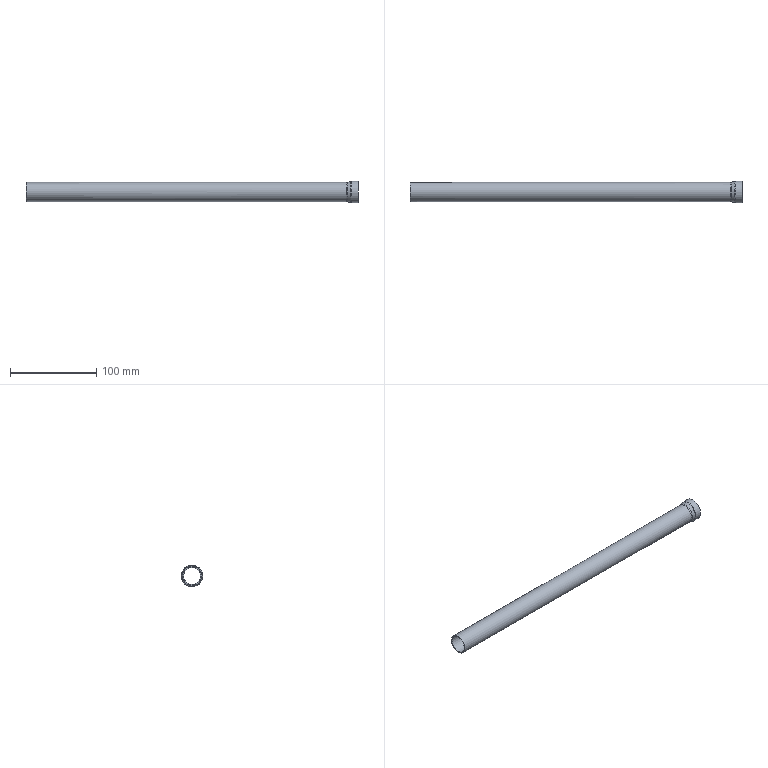Part | NX | features pipe setelah expand 2 | 1 solid | 17 faces | box 385 x 24.9 x 24.9 mm | volume 30600 mm3 | spline 6 | cylinder 4 | torus 3 | plane 2 | cone 2 | commonest cylinder face diameters 19.8 x1 22.2 x1 22.5 x1 24.9 x1
STEP:
#1=CARTESIAN_POINT('',(244.148,128.606,-196.573));
#2=VERTEX_POINT('',#1);
#3=CARTESIAN_POINT('',(244.148,139.394,-176.827));
#4=VERTEX_POINT('',#3);
#5=CARTESIAN_POINT('',(244.148,134.,-186.7));
#6=DIRECTION('',(1.,0.,0.));
#7=DIRECTION('',(0.,1.,0.));
#8=AXIS2_PLACEMENT_3D('',#5,#6,#7);
#9=CIRCLE('',#8,11.25);
#10=EDGE_CURVE('',#2,#4,#9,.T.);
#11=ORIENTED_EDGE('',*,*,#10,.F.);
#12=CARTESIAN_POINT('',(244.148,134.,-186.7));
#13=DIRECTION('',(1.,0.,0.));
#14=DIRECTION('',(0.,1.,0.));
#15=AXIS2_PLACEMENT_3D('',#12,#13,#14);
#16=CIRCLE('',#15,11.25);
#17=EDGE_CURVE('',#4,#2,#16,.T.);
#18=ORIENTED_EDGE('',*,*,#17,.F.);
#19=EDGE_LOOP('',(#11,#18));
#20=FACE_BOUND('',#19,.T.);
#21=CARTESIAN_POINT('',(251.75,134.,-175.45));
#22=VERTEX_POINT('',#21);
#23=CARTESIAN_POINT('',(251.75,134.,-186.7));
#24=DIRECTION('',(-1.,0.,0.));
#25=DIRECTION('',(0.,0.,1.));
#26=AXIS2_PLACEMENT_3D('',#23,#24,#25);
#27=CIRCLE('',#26,11.25);
#28=EDGE_CURVE('',#22,#22,#27,.F.);
#29=ORIENTED_EDGE('',*,*,#28,.T.);
#30=EDGE_LOOP('',(#29));
#31=FACE_BOUND('',#30,.T.);
#32=CARTESIAN_POINT('',(251.75,134.,-186.7));
#33=DIRECTION('',(-1.,0.,0.));
#34=DIRECTION('',(0.,0.,1.));
#35=AXIS2_PLACEMENT_3D('',#32,#33,#34);
#36=CYLINDRICAL_SURFACE('',#35,11.25);
#37=ADVANCED_FACE('',(#20,#31),#36,.F.);
#38=CARTESIAN_POINT('',(243.679,139.364,-176.882));
#39=VERTEX_POINT('',#38);
#40=CARTESIAN_POINT('',(243.679,128.636,-196.518));
#41=VERTEX_POINT('',#40);
#42=CARTESIAN_POINT('',(243.679,134.,-186.7));
#43=DIRECTION('',(1.,0.,0.));
#44=DIRECTION('',(0.,1.,0.));
#45=AXIS2_PLACEMENT_3D('',#42,#43,#44);
#46=CIRCLE('',#45,11.188);
#47=EDGE_CURVE('',#39,#41,#46,.F.);
#48=ORIENTED_EDGE('',*,*,#47,.T.);
#49=CARTESIAN_POINT('',(243.679,128.636,-196.518));
#50=CARTESIAN_POINT('',(243.848,128.614,-196.558));
#51=CARTESIAN_POINT('',(244.006,128.606,-196.573));
#52=CARTESIAN_POINT('',(244.148,128.606,-196.573));
#53=B_SPLINE_CURVE_WITH_KNOTS('',3,(#49,#50,#51,#52),.UNSPECIFIED.,.F.,.F.,(4,4),(0.,1.),.UNSPECIFIED.);
#54=EDGE_CURVE('',#2,#41,#53,.F.);
#55=ORIENTED_EDGE('',*,*,#54,.F.);
#56=ORIENTED_EDGE('',*,*,#10,.T.);
#57=CARTESIAN_POINT('',(244.148,139.394,-176.827));
#58=CARTESIAN_POINT('',(244.006,139.394,-176.827));
#59=CARTESIAN_POINT('',(243.848,139.386,-176.842));
#60=CARTESIAN_POINT('',(243.679,139.364,-176.882));
#61=B_SPLINE_CURVE_WITH_KNOTS('',3,(#57,#58,#59,#60),.UNSPECIFIED.,.F.,.F.,(4,4),(0.,1.),.UNSPECIFIED.);
#62=EDGE_CURVE('',#39,#4,#61,.F.);
#63=ORIENTED_EDGE('',*,*,#62,.F.);
#64=EDGE_LOOP('',(#48,#55,#56,#63));
#65=FACE_BOUND('',#64,.T.);
#66=CARTESIAN_POINT('',(244.148,139.394,-176.827));
#67=CARTESIAN_POINT('',(244.148,159.139,-187.614));
#68=CARTESIAN_POINT('',(244.148,148.352,-207.36));
#69=CARTESIAN_POINT('',(244.148,128.606,-196.573));
#70=CARTESIAN_POINT('',(243.995,139.394,-176.827));
#71=CARTESIAN_POINT('',(243.995,159.139,-187.614));
#72=CARTESIAN_POINT('',(243.995,148.352,-207.36));
#73=CARTESIAN_POINT('',(243.995,128.606,-196.573));
#74=CARTESIAN_POINT('',(243.837,139.384,-176.844));
#75=CARTESIAN_POINT('',(243.837,159.096,-187.613));
#76=CARTESIAN_POINT('',(243.837,148.327,-207.324));
#77=CARTESIAN_POINT('',(243.837,128.616,-196.556));
#78=CARTESIAN_POINT('',(243.679,139.364,-176.882));
#79=CARTESIAN_POINT('',(243.679,159.,-187.609));
#80=CARTESIAN_POINT('',(243.679,148.273,-207.246));
#81=CARTESIAN_POINT('',(243.679,128.636,-196.518));
#82=(BOUNDED_SURFACE()B_SPLINE_SURFACE(3,3,((#66,#67,#68,#69),(#70,#71,#72,#73),(#74,#75,#76,#77),(#78,#79,#80,#81)),.SURF_OF_REVOLUTION.,.F.,.F.,.F.)B_SPLINE_SURFACE_WITH_KNOTS((4,4),(4,4),(0.,0.05912),(0.,1.),.PIECEWISE_BEZIER_KNOTS.)GEOMETRIC_REPRESENTATION_ITEM()RATIONAL_B_SPLINE_SURFACE(((1.,0.3333,0.3333,1.),(0.9264,0.3088,0.3088,0.9264),(0.8614,0.2871,0.2871,0.8614),(0.8052,0.2684,0.2684,0.8052)))REPRESENTATION_ITEM('')SURFACE());
#83=ADVANCED_FACE('',(#65),#82,.T.);
#84=ORIENTED_EDGE('',*,*,#17,.T.);
#85=ORIENTED_EDGE('',*,*,#54,.T.);
#86=CARTESIAN_POINT('',(243.679,134.,-186.7));
#87=DIRECTION('',(1.,0.,0.));
#88=DIRECTION('',(0.,1.,0.));
#89=AXIS2_PLACEMENT_3D('',#86,#87,#88);
#90=CIRCLE('',#89,11.188);
#91=EDGE_CURVE('',#41,#39,#90,.F.);
#92=ORIENTED_EDGE('',*,*,#91,.T.);
#93=ORIENTED_EDGE('',*,*,#62,.T.);
#94=EDGE_LOOP('',(#84,#85,#92,#93));
#95=FACE_BOUND('',#94,.T.);
#96=CARTESIAN_POINT('',(243.679,139.364,-176.882));
#97=CARTESIAN_POINT('',(243.679,119.727,-166.154));
#98=CARTESIAN_POINT('',(243.679,109.,-185.791));
#99=CARTESIAN_POINT('',(243.679,128.636,-196.518));
#100=CARTESIAN_POINT('',(243.826,139.383,-176.847));
#101=CARTESIAN_POINT('',(243.826,119.676,-166.081));
#102=CARTESIAN_POINT('',(243.826,108.911,-185.788));
#103=CARTESIAN_POINT('',(243.826,128.617,-196.553));
#104=CARTESIAN_POINT('',(243.984,139.394,-176.827));
#105=CARTESIAN_POINT('',(243.984,119.648,-166.04));
#106=CARTESIAN_POINT('',(243.984,108.861,-185.786));
#107=CARTESIAN_POINT('',(243.984,128.606,-196.573));
#108=CARTESIAN_POINT('',(244.148,139.394,-176.827));
#109=CARTESIAN_POINT('',(244.148,119.648,-166.04));
#110=CARTESIAN_POINT('',(244.148,108.861,-185.786));
#111=CARTESIAN_POINT('',(244.148,128.606,-196.573));
#112=(BOUNDED_SURFACE()B_SPLINE_SURFACE(3,3,((#96,#97,#98,#99),(#100,#101,#102,#103),(#104,#105,#106,#107),(#108,#109,#110,#111)),.SURF_OF_REVOLUTION.,.F.,.F.,.F.)B_SPLINE_SURFACE_WITH_KNOTS((4,4),(4,4),(0.,0.05912),(0.,1.),.PIECEWISE_BEZIER_KNOTS.)GEOMETRIC_REPRESENTATION_ITEM()RATIONAL_B_SPLINE_SURFACE(((1.,0.3333,0.3333,1.),(0.9264,0.3088,0.3088,0.9264),(0.8614,0.2871,0.2871,0.8614),(0.8052,0.2684,0.2684,0.8052)))REPRESENTATION_ITEM('')SURFACE());
#113=ADVANCED_FACE('',(#95),#112,.T.);
#114=CARTESIAN_POINT('',(251.75,134.,-174.25));
#115=VERTEX_POINT('',#114);
#116=CARTESIAN_POINT('',(251.75,134.,-186.7));
#117=DIRECTION('',(-1.,0.,0.));
#118=DIRECTION('',(0.,0.,1.));
#119=AXIS2_PLACEMENT_3D('',#116,#117,#118);
#120=CIRCLE('',#119,12.45);
#121=EDGE_CURVE('',#115,#115,#120,.T.);
#122=ORIENTED_EDGE('',*,*,#121,.F.);
#123=EDGE_LOOP('',(#122));
#124=FACE_BOUND('',#123,.T.);
#125=ORIENTED_EDGE('',*,*,#28,.F.);
#126=EDGE_LOOP('',(#125));
#127=FACE_BOUND('',#126,.T.);
#128=CARTESIAN_POINT('',(251.75,145.1,-186.7));
#129=DIRECTION('',(-1.,0.,0.));
#130=DIRECTION('',(0.,-1.,0.));
#131=AXIS2_PLACEMENT_3D('',#128,#129,#130);
#132=PLANE('',#131);
#133=ADVANCED_FACE('',(#124,#127),#132,.F.);
#134=CARTESIAN_POINT('',(239.703,123.886,-186.7));
#135=VERTEX_POINT('',#134);
#136=CARTESIAN_POINT('',(239.703,129.151,-195.576));
#137=VERTEX_POINT('',#136);
#138=CARTESIAN_POINT('',(239.703,134.,-186.7));
#139=DIRECTION('',(-1.,0.,0.));
#140=DIRECTION('',(0.,0.,1.));
#141=AXIS2_PLACEMENT_3D('',#138,#139,#140);
#142=CIRCLE('',#141,10.114);
#143=EDGE_CURVE('',#135,#137,#142,.T.);
#144=ORIENTED_EDGE('',*,*,#143,.T.);
#145=CARTESIAN_POINT('',(239.703,134.,-186.7));
#146=DIRECTION('',(-1.,0.,0.));
#147=DIRECTION('',(0.,0.,1.));
#148=AXIS2_PLACEMENT_3D('',#145,#146,#147);
#149=CIRCLE('',#148,10.114);
#150=EDGE_CURVE('',#137,#135,#149,.T.);
#151=ORIENTED_EDGE('',*,*,#150,.T.);
#152=EDGE_LOOP('',(#144,#151));
#153=FACE_BOUND('',#152,.T.);
#154=ORIENTED_EDGE('',*,*,#91,.F.);
#155=ORIENTED_EDGE('',*,*,#47,.F.);
#156=EDGE_LOOP('',(#154,#155));
#157=FACE_BOUND('',#156,.T.);
#158=CARTESIAN_POINT('',(243.679,134.,-186.7));
#159=DIRECTION('',(1.,0.,0.));
#160=DIRECTION('',(0.,0.,-1.));
#161=AXIS2_PLACEMENT_3D('',#158,#159,#160);
#162=CONICAL_SURFACE('',#161,11.188,0.2637);
#163=ADVANCED_FACE('',(#153,#157),#162,.F.);
#164=CARTESIAN_POINT('',(244.148,128.031,-197.626));
#165=VERTEX_POINT('',#164);
#166=CARTESIAN_POINT('',(244.148,139.969,-175.774));
#167=VERTEX_POINT('',#166);
#168=CARTESIAN_POINT('',(244.148,134.,-186.7));
#169=DIRECTION('',(1.,0.,0.));
#170=DIRECTION('',(0.,0.,-1.));
#171=AXIS2_PLACEMENT_3D('',#168,#169,#170);
#172=CIRCLE('',#171,12.45);
#173=EDGE_CURVE('',#165,#167,#172,.T.);
#174=ORIENTED_EDGE('',*,*,#173,.T.);
#175=CARTESIAN_POINT('',(244.148,134.,-186.7));
#176=DIRECTION('',(1.,0.,0.));
#177=DIRECTION('',(0.,0.,-1.));
#178=AXIS2_PLACEMENT_3D('',#175,#176,#177);
#179=CIRCLE('',#178,12.45);
#180=EDGE_CURVE('',#167,#165,#179,.T.);
#181=ORIENTED_EDGE('',*,*,#180,.T.);
#182=EDGE_LOOP('',(#174,#181));
#183=FACE_BOUND('',#182,.T.);
#184=ORIENTED_EDGE('',*,*,#121,.T.);
#185=EDGE_LOOP('',(#184));
#186=FACE_BOUND('',#185,.T.);
#187=CARTESIAN_POINT('',(251.75,134.,-186.7));
#188=DIRECTION('',(-1.,0.,0.));
#189=DIRECTION('',(0.,0.,1.));
#190=AXIS2_PLACEMENT_3D('',#187,#188,#189);
#191=CYLINDRICAL_SURFACE('',#190,12.45);
#192=ADVANCED_FACE('',(#183,#186),#191,.T.);
#193=CARTESIAN_POINT('',(238.087,124.1,-186.7));
#194=VERTEX_POINT('',#193);
#195=CARTESIAN_POINT('',(238.087,117.9,-186.7));
#196=DIRECTION('',(0.,0.000000005,-1.));
#197=DIRECTION('',(0.,1.,0.000000005));
#198=AXIS2_PLACEMENT_3D('',#195,#196,#197);
#199=CIRCLE('',#198,6.2);
#200=EDGE_CURVE('',#194,#135,#199,.T.);
#201=ORIENTED_EDGE('',*,*,#200,.T.);
#202=ORIENTED_EDGE('',*,*,#150,.F.);
#203=CARTESIAN_POINT('',(238.087,129.254,-195.388));
#204=VERTEX_POINT('',#203);
#205=CARTESIAN_POINT('',(238.087,126.281,-200.829));
#206=DIRECTION('',(0.,0.8776,-0.4794));
#207=DIRECTION('',(0.,0.4794,0.8776));
#208=AXIS2_PLACEMENT_3D('',#205,#206,#207);
#209=CIRCLE('',#208,6.2);
#210=EDGE_CURVE('',#137,#204,#209,.F.);
#211=ORIENTED_EDGE('',*,*,#210,.T.);
#212=CARTESIAN_POINT('',(238.087,134.,-186.7));
#213=DIRECTION('',(-1.,0.,0.));
#214=DIRECTION('',(0.,0.,1.));
#215=AXIS2_PLACEMENT_3D('',#212,#213,#214);
#216=CIRCLE('',#215,9.9);
#217=EDGE_CURVE('',#204,#194,#216,.T.);
#218=ORIENTED_EDGE('',*,*,#217,.T.);
#219=EDGE_LOOP('',(#201,#202,#211,#218));
#220=FACE_BOUND('',#219,.T.);
#221=CARTESIAN_POINT('',(238.087,129.254,-195.388));
#222=CARTESIAN_POINT('',(238.087,125.995,-193.608));
#223=CARTESIAN_POINT('',(238.087,124.1,-190.414));
#224=CARTESIAN_POINT('',(238.087,124.1,-186.7));
#225=CARTESIAN_POINT('',(238.613,129.254,-195.388));
#226=CARTESIAN_POINT('',(238.613,125.995,-193.608));
#227=CARTESIAN_POINT('',(238.613,124.1,-190.414));
#228=CARTESIAN_POINT('',(238.613,124.1,-186.7));
#229=CARTESIAN_POINT('',(239.156,129.222,-195.447));
#230=CARTESIAN_POINT('',(239.156,125.941,-193.654));
#231=CARTESIAN_POINT('',(239.156,124.033,-190.439));
#232=CARTESIAN_POINT('',(239.156,124.033,-186.7));
#233=CARTESIAN_POINT('',(239.703,129.151,-195.576));
#234=CARTESIAN_POINT('',(239.703,125.821,-193.757));
#235=CARTESIAN_POINT('',(239.703,123.886,-190.494));
#236=CARTESIAN_POINT('',(239.703,123.886,-186.7));
#237=(BOUNDED_SURFACE()B_SPLINE_SURFACE(3,3,((#221,#222,#223,#224),(#225,#226,#227,#228),(#229,#230,#231,#232),(#233,#234,#235,#236)),.SURF_OF_REVOLUTION.,.F.,.F.,.F.)B_SPLINE_SURFACE_WITH_KNOTS((4,4),(4,4),(0.,0.05912),(0.,1.),.PIECEWISE_BEZIER_KNOTS.)GEOMETRIC_REPRESENTATION_ITEM()RATIONAL_B_SPLINE_SURFACE(((1.,0.9067,0.9067,1.),(0.9264,0.8399,0.8399,0.9264),(0.8614,0.7811,0.7811,0.8614),(0.8052,0.7301,0.7301,0.8052)))REPRESENTATION_ITEM('')SURFACE());
#238=ADVANCED_FACE('',(#220),#237,.F.);
#239=ORIENTED_EDGE('',*,*,#143,.F.);
#240=ORIENTED_EDGE('',*,*,#200,.F.);
#241=CARTESIAN_POINT('',(238.087,134.,-186.7));
#242=DIRECTION('',(-1.,0.,0.));
#243=DIRECTION('',(0.,0.,1.));
#244=AXIS2_PLACEMENT_3D('',#241,#242,#243);
#245=CIRCLE('',#244,9.9);
#246=EDGE_CURVE('',#194,#204,#245,.T.);
#247=ORIENTED_EDGE('',*,*,#246,.T.);
#248=ORIENTED_EDGE('',*,*,#210,.F.);
#249=EDGE_LOOP('',(#239,#240,#247,#248));
#250=FACE_BOUND('',#249,.T.);
#251=CARTESIAN_POINT('',(238.087,134.,-186.7));
#252=DIRECTION('',(1.,0.,0.));
#253=DIRECTION('',(0.,0.,-1.));
#254=AXIS2_PLACEMENT_3D('',#251,#252,#253);
#255=TOROIDAL_SURFACE('',#254,16.1,6.2);
#256=ADVANCED_FACE('',(#250),#255,.T.);
#257=CARTESIAN_POINT('',(243.366,139.919,-175.865));
#258=VERTEX_POINT('',#257);
#259=CARTESIAN_POINT('',(243.366,128.081,-197.535));
#260=VERTEX_POINT('',#259);
#261=CARTESIAN_POINT('',(243.366,134.,-186.7));
#262=DIRECTION('',(1.,0.,0.));
#263=DIRECTION('',(0.,0.,-1.));
#264=AXIS2_PLACEMENT_3D('',#261,#262,#263);
#265=CIRCLE('',#264,12.346);
#266=EDGE_CURVE('',#258,#260,#265,.F.);
#267=ORIENTED_EDGE('',*,*,#266,.F.);
#268=CARTESIAN_POINT('',(244.148,138.531,-178.407));
#269=DIRECTION('',(0.,0.8776,-0.4794));
#270=DIRECTION('',(0.,0.4794,0.8776));
#271=AXIS2_PLACEMENT_3D('',#268,#269,#270);
#272=CIRCLE('',#271,3.);
#273=EDGE_CURVE('',#258,#167,#272,.T.);
#274=ORIENTED_EDGE('',*,*,#273,.T.);
#275=ORIENTED_EDGE('',*,*,#173,.F.);
#276=CARTESIAN_POINT('',(244.148,129.469,-194.993));
#277=DIRECTION('',(0.,0.8776,-0.4794));
#278=DIRECTION('',(0.,0.4794,0.8776));
#279=AXIS2_PLACEMENT_3D('',#276,#277,#278);
#280=CIRCLE('',#279,3.);
#281=EDGE_CURVE('',#165,#260,#280,.T.);
#282=ORIENTED_EDGE('',*,*,#281,.T.);
#283=EDGE_LOOP('',(#267,#274,#275,#282));
#284=FACE_BOUND('',#283,.T.);
#285=CARTESIAN_POINT('',(244.148,139.969,-175.774));
#286=CARTESIAN_POINT('',(244.148,161.821,-187.712));
#287=CARTESIAN_POINT('',(244.148,149.883,-209.564));
#288=CARTESIAN_POINT('',(244.148,128.031,-197.626));
#289=CARTESIAN_POINT('',(243.893,139.969,-175.774));
#290=CARTESIAN_POINT('',(243.893,161.821,-187.712));
#291=CARTESIAN_POINT('',(243.893,149.883,-209.564));
#292=CARTESIAN_POINT('',(243.893,128.031,-197.626));
#293=CARTESIAN_POINT('',(243.63,139.953,-175.802));
#294=CARTESIAN_POINT('',(243.63,161.748,-187.709));
#295=CARTESIAN_POINT('',(243.63,149.842,-209.504));
#296=CARTESIAN_POINT('',(243.63,128.047,-197.598));
#297=CARTESIAN_POINT('',(243.366,139.919,-175.865));
#298=CARTESIAN_POINT('',(243.366,161.589,-187.703));
#299=CARTESIAN_POINT('',(243.366,149.751,-209.373));
#300=CARTESIAN_POINT('',(243.366,128.081,-197.535));
#301=(BOUNDED_SURFACE()B_SPLINE_SURFACE(3,3,((#285,#286,#287,#288),(#289,#290,#291,#292),(#293,#294,#295,#296),(#297,#298,#299,#300)),.SURF_OF_REVOLUTION.,.F.,.F.,.F.)B_SPLINE_SURFACE_WITH_KNOTS((4,4),(4,4),(0.,0.05912),(0.,1.),.PIECEWISE_BEZIER_KNOTS.)GEOMETRIC_REPRESENTATION_ITEM()RATIONAL_B_SPLINE_SURFACE(((1.,0.3333,0.3333,1.),(0.9264,0.3088,0.3088,0.9264),(0.8614,0.2871,0.2871,0.8614),(0.8052,0.2684,0.2684,0.8052)))REPRESENTATION_ITEM('')SURFACE());
#302=ADVANCED_FACE('',(#284),#301,.F.);
#303=CARTESIAN_POINT('',(243.366,134.,-186.7));
#304=DIRECTION('',(1.,0.,0.));
#305=DIRECTION('',(0.,0.,-1.));
#306=AXIS2_PLACEMENT_3D('',#303,#304,#305);
#307=CIRCLE('',#306,12.346);
#308=EDGE_CURVE('',#260,#258,#307,.F.);
#309=ORIENTED_EDGE('',*,*,#308,.F.);
#310=ORIENTED_EDGE('',*,*,#281,.F.);
#311=ORIENTED_EDGE('',*,*,#180,.F.);
#312=ORIENTED_EDGE('',*,*,#273,.F.);
#313=EDGE_LOOP('',(#309,#310,#311,#312));
#314=FACE_BOUND('',#313,.T.);
#315=CARTESIAN_POINT('',(244.148,134.,-186.7));
#316=DIRECTION('',(1.,0.,0.));
#317=DIRECTION('',(0.,1.,0.));
#318=AXIS2_PLACEMENT_3D('',#315,#316,#317);
#319=TOROIDAL_SURFACE('',#318,9.45,3.);
#320=ADVANCED_FACE('',(#314),#319,.T.);
#321=ORIENTED_EDGE('',*,*,#246,.F.);
#322=ORIENTED_EDGE('',*,*,#217,.F.);
#323=EDGE_LOOP('',(#321,#322));
#324=FACE_BOUND('',#323,.T.);
#325=CARTESIAN_POINT('',(-133.25,134.,-176.8));
#326=VERTEX_POINT('',#325);
#327=CARTESIAN_POINT('',(-133.25,134.,-186.7));
#328=DIRECTION('',(-1.,0.,0.));
#329=DIRECTION('',(0.,0.,1.));
#330=AXIS2_PLACEMENT_3D('',#327,#328,#329);
#331=CIRCLE('',#330,9.9);
#332=EDGE_CURVE('',#326,#326,#331,.T.);
#333=ORIENTED_EDGE('',*,*,#332,.T.);
#334=EDGE_LOOP('',(#333));
#335=FACE_BOUND('',#334,.T.);
#336=CARTESIAN_POINT('',(238.087,134.,-186.7));
#337=DIRECTION('',(-1.,0.,0.));
#338=DIRECTION('',(0.,0.,1.));
#339=AXIS2_PLACEMENT_3D('',#336,#337,#338);
#340=CYLINDRICAL_SURFACE('',#339,9.9);
#341=ADVANCED_FACE('',(#324,#335),#340,.F.);
#342=CARTESIAN_POINT('',(239.39,145.273,-186.7));
#343=VERTEX_POINT('',#342);
#344=CARTESIAN_POINT('',(238.087,145.1,-186.7));
#345=VERTEX_POINT('',#344);
#346=CARTESIAN_POINT('',(238.087,150.1,-186.7));
#347=DIRECTION('',(0.,0.000000004,-1.));
#348=DIRECTION('',(0.,1.,0.000000004));
#349=AXIS2_PLACEMENT_3D('',#346,#347,#348);
#350=CIRCLE('',#349,5.);
#351=EDGE_CURVE('',#343,#345,#350,.T.);
#352=ORIENTED_EDGE('',*,*,#351,.T.);
#353=CARTESIAN_POINT('',(238.087,122.9,-186.7));
#354=VERTEX_POINT('',#353);
#355=CARTESIAN_POINT('',(238.087,134.,-186.7));
#356=DIRECTION('',(-1.,0.,0.));
#357=DIRECTION('',(0.,0.,1.));
#358=AXIS2_PLACEMENT_3D('',#355,#356,#357);
#359=CIRCLE('',#358,11.1);
#360=EDGE_CURVE('',#354,#345,#359,.T.);
#361=ORIENTED_EDGE('',*,*,#360,.F.);
#362=CARTESIAN_POINT('',(239.39,122.727,-186.7));
#363=VERTEX_POINT('',#362);
#364=CARTESIAN_POINT('',(238.087,117.9,-186.7));
#365=DIRECTION('',(0.,0.000000004,-1.));
#366=DIRECTION('',(0.,1.,0.000000004));
#367=AXIS2_PLACEMENT_3D('',#364,#365,#366);
#368=CIRCLE('',#367,5.);
#369=EDGE_CURVE('',#354,#363,#368,.T.);
#370=ORIENTED_EDGE('',*,*,#369,.T.);
#371=CARTESIAN_POINT('',(239.39,134.,-186.7));
#372=DIRECTION('',(1.,0.,0.));
#373=DIRECTION('',(0.,0.,-1.));
#374=AXIS2_PLACEMENT_3D('',#371,#372,#373);
#375=CIRCLE('',#374,11.273);
#376=EDGE_CURVE('',#343,#363,#375,.T.);
#377=ORIENTED_EDGE('',*,*,#376,.F.);
#378=EDGE_LOOP('',(#352,#361,#370,#377));
#379=FACE_BOUND('',#378,.T.);
#380=CARTESIAN_POINT('',(238.087,134.,-186.7));
#381=DIRECTION('',(-1.,0.,0.));
#382=DIRECTION('',(0.,0.,1.));
#383=AXIS2_PLACEMENT_3D('',#380,#381,#382);
#384=TOROIDAL_SURFACE('',#383,16.1,5.);
#385=ADVANCED_FACE('',(#379),#384,.F.);
#386=ORIENTED_EDGE('',*,*,#308,.T.);
#387=ORIENTED_EDGE('',*,*,#266,.T.);
#388=EDGE_LOOP('',(#386,#387));
#389=FACE_BOUND('',#388,.T.);
#390=CARTESIAN_POINT('',(239.39,128.596,-196.593));
#391=VERTEX_POINT('',#390);
#392=CARTESIAN_POINT('',(239.39,134.,-186.7));
#393=DIRECTION('',(-1.,0.,0.));
#394=DIRECTION('',(0.,0.,1.));
#395=AXIS2_PLACEMENT_3D('',#392,#393,#394);
#396=CIRCLE('',#395,11.273);
#397=EDGE_CURVE('',#343,#391,#396,.T.);
#398=ORIENTED_EDGE('',*,*,#397,.F.);
#399=ORIENTED_EDGE('',*,*,#376,.T.);
#400=CARTESIAN_POINT('',(239.39,134.,-186.7));
#401=DIRECTION('',(-1.,0.,0.));
#402=DIRECTION('',(0.,0.,1.));
#403=AXIS2_PLACEMENT_3D('',#400,#401,#402);
#404=CIRCLE('',#403,11.273);
#405=EDGE_CURVE('',#391,#363,#404,.T.);
#406=ORIENTED_EDGE('',*,*,#405,.F.);
#407=EDGE_LOOP('',(#398,#399,#406));
#408=FACE_BOUND('',#407,.T.);
#409=CARTESIAN_POINT('',(243.366,134.,-186.7));
#410=DIRECTION('',(1.,0.,0.));
#411=DIRECTION('',(0.,1.,0.));
#412=AXIS2_PLACEMENT_3D('',#409,#410,#411);
#413=CONICAL_SURFACE('',#412,12.346,0.2637);
#414=ADVANCED_FACE('',(#389,#408),#413,.T.);
#415=CARTESIAN_POINT('',(-133.25,134.,-175.6));
#416=VERTEX_POINT('',#415);
#417=CARTESIAN_POINT('',(-133.25,134.,-186.7));
#418=DIRECTION('',(-1.,0.,0.));
#419=DIRECTION('',(0.,0.,1.));
#420=AXIS2_PLACEMENT_3D('',#417,#418,#419);
#421=CIRCLE('',#420,11.1);
#422=EDGE_CURVE('',#416,#416,#421,.F.);
#423=ORIENTED_EDGE('',*,*,#422,.F.);
#424=EDGE_LOOP('',(#423));
#425=FACE_BOUND('',#424,.T.);
#426=ORIENTED_EDGE('',*,*,#332,.F.);
#427=EDGE_LOOP('',(#426));
#428=FACE_BOUND('',#427,.T.);
#429=CARTESIAN_POINT('',(-133.25,0.,0.));
#430=DIRECTION('',(1.,0.,0.));
#431=DIRECTION('',(0.,1.,0.));
#432=AXIS2_PLACEMENT_3D('',#429,#430,#431);
#433=PLANE('',#432);
#434=ADVANCED_FACE('',(#425,#428),#433,.F.);
#435=CARTESIAN_POINT('',(238.087,128.678,-196.441));
#436=VERTEX_POINT('',#435);
#437=CARTESIAN_POINT('',(239.39,128.596,-196.593));
#438=CARTESIAN_POINT('',(238.919,128.657,-196.481));
#439=CARTESIAN_POINT('',(238.48,128.678,-196.441));
#440=CARTESIAN_POINT('',(238.087,128.678,-196.441));
#441=B_SPLINE_CURVE_WITH_KNOTS('',3,(#437,#438,#439,#440),.UNSPECIFIED.,.F.,.F.,(4,4),(0.,1.),.UNSPECIFIED.);
#442=EDGE_CURVE('',#436,#391,#441,.F.);
#443=ORIENTED_EDGE('',*,*,#442,.F.);
#444=CARTESIAN_POINT('',(238.087,134.,-186.7));
#445=DIRECTION('',(-1.,0.,0.));
#446=DIRECTION('',(0.,0.,1.));
#447=AXIS2_PLACEMENT_3D('',#444,#445,#446);
#448=CIRCLE('',#447,11.1);
#449=EDGE_CURVE('',#345,#436,#448,.T.);
#450=ORIENTED_EDGE('',*,*,#449,.F.);
#451=ORIENTED_EDGE('',*,*,#351,.F.);
#452=ORIENTED_EDGE('',*,*,#397,.T.);
#453=EDGE_LOOP('',(#443,#450,#451,#452));
#454=FACE_BOUND('',#453,.T.);
#455=CARTESIAN_POINT('',(238.087,145.1,-186.7));
#456=CARTESIAN_POINT('',(238.087,145.1,-196.15));
#457=CARTESIAN_POINT('',(238.087,136.972,-200.972));
#458=CARTESIAN_POINT('',(238.087,128.678,-196.441));
#459=CARTESIAN_POINT('',(238.511,145.1,-186.7));
#460=CARTESIAN_POINT('',(238.511,145.1,-196.15));
#461=CARTESIAN_POINT('',(238.511,136.972,-200.972));
#462=CARTESIAN_POINT('',(238.511,128.678,-196.441));
#463=CARTESIAN_POINT('',(238.949,145.154,-186.7));
#464=CARTESIAN_POINT('',(238.949,145.154,-196.196));
#465=CARTESIAN_POINT('',(238.949,136.986,-201.041));
#466=CARTESIAN_POINT('',(238.949,128.653,-196.488));
#467=CARTESIAN_POINT('',(239.39,145.273,-186.7));
#468=CARTESIAN_POINT('',(239.39,145.273,-196.298));
#469=CARTESIAN_POINT('',(239.39,137.018,-201.194));
#470=CARTESIAN_POINT('',(239.39,128.596,-196.593));
#471=(BOUNDED_SURFACE()B_SPLINE_SURFACE(3,3,((#455,#456,#457,#458),(#459,#460,#461,#462),(#463,#464,#465,#466),(#467,#468,#469,#470)),.SURF_OF_REVOLUTION.,.F.,.F.,.F.)B_SPLINE_SURFACE_WITH_KNOTS((4,4),(4,4),(0.,0.05912),(0.,1.),.PIECEWISE_BEZIER_KNOTS.)GEOMETRIC_REPRESENTATION_ITEM()RATIONAL_B_SPLINE_SURFACE(((1.,0.6735,0.6735,1.),(0.9264,0.6239,0.6239,0.9264),(0.8614,0.5801,0.5801,0.8614),(0.8052,0.5423,0.5423,0.8052)))REPRESENTATION_ITEM('')SURFACE());
#472=ADVANCED_FACE('',(#454),#471,.T.);
#473=ORIENTED_EDGE('',*,*,#369,.F.);
#474=CARTESIAN_POINT('',(238.087,134.,-186.7));
#475=DIRECTION('',(-1.,0.,0.));
#476=DIRECTION('',(0.,0.,1.));
#477=AXIS2_PLACEMENT_3D('',#474,#475,#476);
#478=CIRCLE('',#477,11.1);
#479=EDGE_CURVE('',#436,#354,#478,.T.);
#480=ORIENTED_EDGE('',*,*,#479,.F.);
#481=ORIENTED_EDGE('',*,*,#442,.T.);
#482=ORIENTED_EDGE('',*,*,#405,.T.);
#483=EDGE_LOOP('',(#473,#480,#481,#482));
#484=FACE_BOUND('',#483,.T.);
#485=CARTESIAN_POINT('',(238.087,128.678,-196.441));
#486=CARTESIAN_POINT('',(238.087,125.024,-194.445));
#487=CARTESIAN_POINT('',(238.087,122.9,-190.864));
#488=CARTESIAN_POINT('',(238.087,122.9,-186.7));
#489=CARTESIAN_POINT('',(238.511,128.678,-196.441));
#490=CARTESIAN_POINT('',(238.511,125.024,-194.445));
#491=CARTESIAN_POINT('',(238.511,122.9,-190.864));
#492=CARTESIAN_POINT('',(238.511,122.9,-186.7));
#493=CARTESIAN_POINT('',(238.949,128.653,-196.488));
#494=CARTESIAN_POINT('',(238.949,124.981,-194.483));
#495=CARTESIAN_POINT('',(238.949,122.846,-190.884));
#496=CARTESIAN_POINT('',(238.949,122.846,-186.7));
#497=CARTESIAN_POINT('',(239.39,128.596,-196.593));
#498=CARTESIAN_POINT('',(239.39,124.885,-194.566));
#499=CARTESIAN_POINT('',(239.39,122.727,-190.929));
#500=CARTESIAN_POINT('',(239.39,122.727,-186.7));
#501=(BOUNDED_SURFACE()B_SPLINE_SURFACE(3,3,((#485,#486,#487,#488),(#489,#490,#491,#492),(#493,#494,#495,#496),(#497,#498,#499,#500)),.SURF_OF_REVOLUTION.,.F.,.F.,.F.)B_SPLINE_SURFACE_WITH_KNOTS((4,4),(4,4),(0.,0.05912),(0.,1.),.PIECEWISE_BEZIER_KNOTS.)GEOMETRIC_REPRESENTATION_ITEM()RATIONAL_B_SPLINE_SURFACE(((1.,0.9067,0.9067,1.),(0.9264,0.8399,0.8399,0.9264),(0.8614,0.7811,0.7811,0.8614),(0.8052,0.7301,0.7301,0.8052)))REPRESENTATION_ITEM('')SURFACE());
#502=ADVANCED_FACE('',(#484),#501,.T.);
#503=ORIENTED_EDGE('',*,*,#479,.T.);
#504=ORIENTED_EDGE('',*,*,#360,.T.);
#505=ORIENTED_EDGE('',*,*,#449,.T.);
#506=EDGE_LOOP('',(#503,#504,#505));
#507=FACE_BOUND('',#506,.T.);
#508=ORIENTED_EDGE('',*,*,#422,.T.);
#509=EDGE_LOOP('',(#508));
#510=FACE_BOUND('',#509,.T.);
#511=CARTESIAN_POINT('',(238.087,134.,-186.7));
#512=DIRECTION('',(-1.,0.,0.));
#513=DIRECTION('',(0.,0.,1.));
#514=AXIS2_PLACEMENT_3D('',#511,#512,#513);
#515=CYLINDRICAL_SURFACE('',#514,11.1);
#516=ADVANCED_FACE('',(#507,#510),#515,.T.);
#517=CLOSED_SHELL('',(#37,#83,#113,#133,#163,#192,#238,#256,#302,#320,#341,#385,#414,#434,#472,#502,#516));
#518=MANIFOLD_SOLID_BREP('',#517);
#519=(LENGTH_UNIT()NAMED_UNIT(*)SI_UNIT(.MILLI.,.METRE.));
#520=UNCERTAINTY_MEASURE_WITH_UNIT(LENGTH_MEASURE(0.0508),#519,'','');
#521=(NAMED_UNIT(*)PLANE_ANGLE_UNIT()SI_UNIT($,.RADIAN.));
#522=(NAMED_UNIT(*)SI_UNIT($,.STERADIAN.)SOLID_ANGLE_UNIT());
#523=(GEOMETRIC_REPRESENTATION_CONTEXT(3)GLOBAL_UNCERTAINTY_ASSIGNED_CONTEXT((#520))GLOBAL_UNIT_ASSIGNED_CONTEXT((#519,#521,#522))REPRESENTATION_CONTEXT('',''));
#524=ADVANCED_BREP_SHAPE_REPRESENTATION('',(#518),#523);